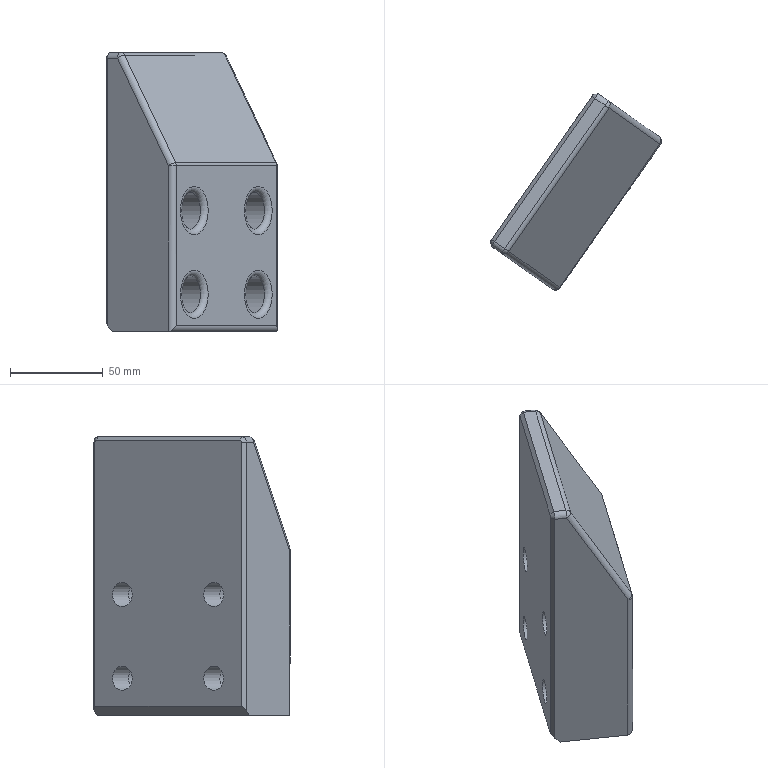Part | NX | features solid 2 | 1 solid | 42 faces | box 91.894 x 105.401 x 150 mm | volume 521981 mm3 | cylinder 17 | plane 15 | torus 4 | sphere 4 | cone 2 | commonest cylinder face diameters 6 x9 13 x4 20 x4
STEP:
#1=CARTESIAN_POINT('',(267.886,524.136,-269.059));
#2=VERTEX_POINT('',#1);
#3=CARTESIAN_POINT('',(260.429,513.487,-269.059));
#4=DIRECTION('',(0.8192,-0.5736,0.));
#5=DIRECTION('',(0.5736,0.8192,0.));
#6=AXIS2_PLACEMENT_3D('',#3,#4,#5);
#7=CIRCLE('',#6,13.);
#8=EDGE_CURVE('',#2,#2,#7,.F.);
#9=ORIENTED_EDGE('',*,*,#8,.T.);
#10=EDGE_LOOP('',(#9));
#11=FACE_BOUND('',#10,.T.);
#12=CARTESIAN_POINT('',(267.886,524.136,-314.059));
#13=VERTEX_POINT('',#12);
#14=CARTESIAN_POINT('',(260.429,513.487,-314.059));
#15=DIRECTION('',(0.8192,-0.5736,0.));
#16=DIRECTION('',(0.5736,0.8192,0.));
#17=AXIS2_PLACEMENT_3D('',#14,#15,#16);
#18=CIRCLE('',#17,13.);
#19=EDGE_CURVE('',#13,#13,#18,.F.);
#20=ORIENTED_EDGE('',*,*,#19,.T.);
#21=EDGE_LOOP('',(#20));
#22=FACE_BOUND('',#21,.T.);
#23=CARTESIAN_POINT('',(233.471,474.987,-269.059));
#24=VERTEX_POINT('',#23);
#25=CARTESIAN_POINT('',(226.015,464.338,-269.059));
#26=DIRECTION('',(0.8192,-0.5736,0.));
#27=DIRECTION('',(0.5736,0.8192,0.));
#28=AXIS2_PLACEMENT_3D('',#25,#26,#27);
#29=CIRCLE('',#28,13.);
#30=EDGE_CURVE('',#24,#24,#29,.F.);
#31=ORIENTED_EDGE('',*,*,#30,.T.);
#32=EDGE_LOOP('',(#31));
#33=FACE_BOUND('',#32,.T.);
#34=CARTESIAN_POINT('',(233.471,474.987,-314.059));
#35=VERTEX_POINT('',#34);
#36=CARTESIAN_POINT('',(226.015,464.338,-314.059));
#37=DIRECTION('',(0.8192,-0.5736,0.));
#38=DIRECTION('',(0.5736,0.8192,0.));
#39=AXIS2_PLACEMENT_3D('',#36,#37,#38);
#40=CIRCLE('',#39,13.);
#41=EDGE_CURVE('',#35,#35,#40,.F.);
#42=ORIENTED_EDGE('',*,*,#41,.T.);
#43=EDGE_LOOP('',(#42));
#44=FACE_BOUND('',#43,.T.);
#45=CARTESIAN_POINT('',(216.264,450.412,-244.863));
#46=VERTEX_POINT('',#45);
#47=CARTESIAN_POINT('',(216.264,450.412,-331.059));
#48=VERTEX_POINT('',#47);
#49=CARTESIAN_POINT('',(216.264,450.412,-334.059));
#50=DIRECTION('',(0.,0.,1.));
#51=VECTOR('',#50,1000.);
#52=LINE('',#49,#51);
#53=EDGE_CURVE('',#46,#48,#52,.F.);
#54=ORIENTED_EDGE('',*,*,#53,.T.);
#55=CARTESIAN_POINT('',(270.18,527.412,-331.059));
#56=VERTEX_POINT('',#55);
#57=CARTESIAN_POINT('',(271.901,529.87,-331.059));
#58=DIRECTION('',(-0.5736,-0.8192,0.));
#59=VECTOR('',#58,1000.);
#60=LINE('',#57,#59);
#61=EDGE_CURVE('',#48,#56,#60,.F.);
#62=ORIENTED_EDGE('',*,*,#61,.T.);
#63=CARTESIAN_POINT('',(270.18,527.412,-244.863));
#64=VERTEX_POINT('',#63);
#65=CARTESIAN_POINT('',(270.18,527.412,-244.059));
#66=DIRECTION('',(0.,0.,1.));
#67=VECTOR('',#66,1000.);
#68=LINE('',#65,#67);
#69=EDGE_CURVE('',#56,#64,#68,.T.);
#70=ORIENTED_EDGE('',*,*,#69,.T.);
#71=CARTESIAN_POINT('',(271.901,529.87,-244.863));
#72=DIRECTION('',(-0.5736,-0.8192,0.));
#73=VECTOR('',#72,1000.);
#74=LINE('',#71,#73);
#75=EDGE_CURVE('',#64,#46,#74,.T.);
#76=ORIENTED_EDGE('',*,*,#75,.T.);
#77=EDGE_LOOP('',(#54,#62,#70,#76));
#78=FACE_BOUND('',#77,.T.);
#79=CARTESIAN_POINT('',(271.901,529.87,-334.059));
#80=DIRECTION('',(0.8192,-0.5736,0.));
#81=DIRECTION('',(0.5736,0.8192,0.));
#82=AXIS2_PLACEMENT_3D('',#79,#80,#81);
#83=PLANE('',#82);
#84=ADVANCED_FACE('',(#11,#22,#33,#44,#78),#83,.T.);
#85=CARTESIAN_POINT('',(269.851,527.643,-243.363));
#86=VERTEX_POINT('',#85);
#87=CARTESIAN_POINT('',(242.513,546.785,-185.559));
#88=VERTEX_POINT('',#87);
#89=CARTESIAN_POINT('',(241.804,547.282,-184.059));
#90=DIRECTION('',(-0.4096,0.2868,0.866));
#91=VECTOR('',#90,1000.);
#92=LINE('',#89,#91);
#93=EDGE_CURVE('',#86,#88,#92,.T.);
#94=ORIENTED_EDGE('',*,*,#93,.T.);
#95=CARTESIAN_POINT('',(188.597,469.785,-185.559));
#96=VERTEX_POINT('',#95);
#97=CARTESIAN_POINT('',(244.234,549.242,-185.559));
#98=DIRECTION('',(-0.5736,-0.8192,0.));
#99=VECTOR('',#98,1000.);
#100=LINE('',#97,#99);
#101=EDGE_CURVE('',#88,#96,#100,.T.);
#102=ORIENTED_EDGE('',*,*,#101,.T.);
#103=CARTESIAN_POINT('',(215.935,450.643,-243.363));
#104=VERTEX_POINT('',#103);
#105=CARTESIAN_POINT('',(216.264,450.412,-244.059));
#106=DIRECTION('',(-0.4096,0.2868,0.866));
#107=VECTOR('',#106,1000.);
#108=LINE('',#105,#107);
#109=EDGE_CURVE('',#96,#104,#108,.F.);
#110=ORIENTED_EDGE('',*,*,#109,.T.);
#111=CARTESIAN_POINT('',(271.572,530.1,-243.363));
#112=DIRECTION('',(-0.5736,-0.8192,0.));
#113=VECTOR('',#112,1000.);
#114=LINE('',#111,#113);
#115=EDGE_CURVE('',#104,#86,#114,.F.);
#116=ORIENTED_EDGE('',*,*,#115,.T.);
#117=EDGE_LOOP('',(#94,#102,#110,#116));
#118=FACE_BOUND('',#117,.T.);
#119=CARTESIAN_POINT('',(271.901,529.87,-244.059));
#120=DIRECTION('',(0.7094,-0.4967,0.5));
#121=DIRECTION('',(0.4096,-0.2868,-0.866));
#122=AXIS2_PLACEMENT_3D('',#119,#120,#121);
#123=PLANE('',#122);
#124=ADVANCED_FACE('',(#118),#123,.T.);
#125=CARTESIAN_POINT('',(240.385,548.275,-184.059));
#126=VERTEX_POINT('',#125);
#127=CARTESIAN_POINT('',(234.957,552.076,-184.059));
#128=VERTEX_POINT('',#127);
#129=CARTESIAN_POINT('',(233.318,553.223,-184.059));
#130=DIRECTION('',(-0.8192,0.5736,0.));
#131=VECTOR('',#130,1000.);
#132=LINE('',#129,#131);
#133=EDGE_CURVE('',#126,#128,#132,.T.);
#134=ORIENTED_EDGE('',*,*,#133,.T.);
#135=CARTESIAN_POINT('',(181.041,475.076,-184.059));
#136=VERTEX_POINT('',#135);
#137=CARTESIAN_POINT('',(236.677,554.534,-184.059));
#138=DIRECTION('',(-0.5736,-0.8192,0.));
#139=VECTOR('',#138,1000.);
#140=LINE('',#137,#139);
#141=EDGE_CURVE('',#128,#136,#140,.T.);
#142=ORIENTED_EDGE('',*,*,#141,.T.);
#143=CARTESIAN_POINT('',(186.469,471.275,-184.059));
#144=VERTEX_POINT('',#143);
#145=CARTESIAN_POINT('',(187.888,470.281,-184.059));
#146=DIRECTION('',(-0.8192,0.5736,0.));
#147=VECTOR('',#146,1000.);
#148=LINE('',#145,#147);
#149=EDGE_CURVE('',#136,#144,#148,.F.);
#150=ORIENTED_EDGE('',*,*,#149,.T.);
#151=CARTESIAN_POINT('',(242.106,550.733,-184.059));
#152=DIRECTION('',(-0.5736,-0.8192,0.));
#153=VECTOR('',#152,1000.);
#154=LINE('',#151,#153);
#155=EDGE_CURVE('',#144,#126,#154,.F.);
#156=ORIENTED_EDGE('',*,*,#155,.T.);
#157=EDGE_LOOP('',(#134,#142,#150,#156));
#158=FACE_BOUND('',#157,.T.);
#159=CARTESIAN_POINT('',(243.525,549.739,-184.059));
#160=DIRECTION('',(0.,0.,1.));
#161=DIRECTION('',(-0.5736,-0.8192,0.));
#162=AXIS2_PLACEMENT_3D('',#159,#160,#161);
#163=PLANE('',#162);
#164=ADVANCED_FACE('',(#158),#163,.T.);
#165=CARTESIAN_POINT('',(219.839,533.973,-269.059));
#166=VERTEX_POINT('',#165);
#167=CARTESIAN_POINT('',(223.568,539.298,-269.059));
#168=DIRECTION('',(-0.8192,0.5736,0.));
#169=DIRECTION('',(-0.5736,-0.8192,0.));
#170=AXIS2_PLACEMENT_3D('',#167,#168,#169);
#171=CIRCLE('',#170,6.5);
#172=EDGE_CURVE('',#166,#166,#171,.T.);
#173=ORIENTED_EDGE('',*,*,#172,.F.);
#174=EDGE_LOOP('',(#173));
#175=FACE_BOUND('',#174,.T.);
#176=CARTESIAN_POINT('',(185.425,484.824,-269.059));
#177=VERTEX_POINT('',#176);
#178=CARTESIAN_POINT('',(189.153,490.149,-269.059));
#179=DIRECTION('',(-0.8192,0.5736,0.));
#180=DIRECTION('',(-0.5736,-0.8192,0.));
#181=AXIS2_PLACEMENT_3D('',#178,#179,#180);
#182=CIRCLE('',#181,6.5);
#183=EDGE_CURVE('',#177,#177,#182,.T.);
#184=ORIENTED_EDGE('',*,*,#183,.F.);
#185=EDGE_LOOP('',(#184));
#186=FACE_BOUND('',#185,.T.);
#187=CARTESIAN_POINT('',(219.839,533.973,-314.059));
#188=VERTEX_POINT('',#187);
#189=CARTESIAN_POINT('',(223.568,539.298,-314.059));
#190=DIRECTION('',(-0.8192,0.5736,0.));
#191=DIRECTION('',(-0.5736,-0.8192,0.));
#192=AXIS2_PLACEMENT_3D('',#189,#190,#191);
#193=CIRCLE('',#192,6.5);
#194=EDGE_CURVE('',#188,#188,#193,.T.);
#195=ORIENTED_EDGE('',*,*,#194,.F.);
#196=EDGE_LOOP('',(#195));
#197=FACE_BOUND('',#196,.T.);
#198=CARTESIAN_POINT('',(185.425,484.824,-314.059));
#199=VERTEX_POINT('',#198);
#200=CARTESIAN_POINT('',(189.153,490.149,-314.059));
#201=DIRECTION('',(-0.8192,0.5736,0.));
#202=DIRECTION('',(-0.5736,-0.8192,0.));
#203=AXIS2_PLACEMENT_3D('',#200,#201,#202);
#204=CIRCLE('',#203,6.5);
#205=EDGE_CURVE('',#199,#199,#204,.T.);
#206=ORIENTED_EDGE('',*,*,#205,.F.);
#207=EDGE_LOOP('',(#206));
#208=FACE_BOUND('',#207,.T.);
#209=CARTESIAN_POINT('',(233.892,554.043,-187.059));
#210=VERTEX_POINT('',#209);
#211=CARTESIAN_POINT('',(233.892,554.043,-329.059));
#212=VERTEX_POINT('',#211);
#213=CARTESIAN_POINT('',(233.892,554.043,-334.059));
#214=DIRECTION('',(0.,0.,-1.));
#215=VECTOR('',#214,1000.);
#216=LINE('',#213,#215);
#217=EDGE_CURVE('',#210,#212,#216,.T.);
#218=ORIENTED_EDGE('',*,*,#217,.T.);
#219=CARTESIAN_POINT('',(178.829,475.404,-329.059));
#220=VERTEX_POINT('',#219);
#221=CARTESIAN_POINT('',(235.039,555.681,-329.059));
#222=DIRECTION('',(-0.5736,-0.8192,0.));
#223=VECTOR('',#222,1000.);
#224=LINE('',#221,#223);
#225=EDGE_CURVE('',#212,#220,#224,.T.);
#226=ORIENTED_EDGE('',*,*,#225,.T.);
#227=CARTESIAN_POINT('',(178.829,475.404,-187.059));
#228=VERTEX_POINT('',#227);
#229=CARTESIAN_POINT('',(178.829,475.404,-184.059));
#230=DIRECTION('',(0.,0.,1.));
#231=VECTOR('',#230,1000.);
#232=LINE('',#229,#231);
#233=EDGE_CURVE('',#220,#228,#232,.T.);
#234=ORIENTED_EDGE('',*,*,#233,.T.);
#235=CARTESIAN_POINT('',(179.402,476.223,-186.059));
#236=VERTEX_POINT('',#235);
#237=CARTESIAN_POINT('',(179.402,476.223,-187.059));
#238=DIRECTION('',(-0.8192,0.5736,0.));
#239=DIRECTION('',(0.,0.,1.));
#240=AXIS2_PLACEMENT_3D('',#237,#238,#239);
#241=CIRCLE('',#240,1.);
#242=EDGE_CURVE('',#228,#236,#241,.T.);
#243=ORIENTED_EDGE('',*,*,#242,.T.);
#244=CARTESIAN_POINT('',(233.318,553.223,-186.059));
#245=VERTEX_POINT('',#244);
#246=CARTESIAN_POINT('',(235.039,555.681,-186.059));
#247=DIRECTION('',(0.5736,0.8192,0.));
#248=VECTOR('',#247,1000.);
#249=LINE('',#246,#248);
#250=EDGE_CURVE('',#236,#245,#249,.T.);
#251=ORIENTED_EDGE('',*,*,#250,.T.);
#252=CARTESIAN_POINT('',(233.318,553.223,-187.059));
#253=DIRECTION('',(-0.8192,0.5736,0.));
#254=DIRECTION('',(0.,0.,1.));
#255=AXIS2_PLACEMENT_3D('',#252,#253,#254);
#256=CIRCLE('',#255,1.);
#257=EDGE_CURVE('',#245,#210,#256,.T.);
#258=ORIENTED_EDGE('',*,*,#257,.T.);
#259=EDGE_LOOP('',(#218,#226,#234,#243,#251,#258));
#260=FACE_BOUND('',#259,.T.);
#261=CARTESIAN_POINT('',(235.039,555.681,-184.059));
#262=DIRECTION('',(-0.8192,0.5736,0.));
#263=DIRECTION('',(0.,0.,1.));
#264=AXIS2_PLACEMENT_3D('',#261,#262,#263);
#265=PLANE('',#264);
#266=ADVANCED_FACE('',(#175,#186,#197,#208,#260),#265,.T.);
#267=CARTESIAN_POINT('',(181.777,470.898,-334.059));
#268=VERTEX_POINT('',#267);
#269=CARTESIAN_POINT('',(212.086,449.675,-334.059));
#270=VERTEX_POINT('',#269);
#271=CARTESIAN_POINT('',(177.682,473.766,-334.059));
#272=DIRECTION('',(0.8192,-0.5736,0.));
#273=VECTOR('',#272,1000.);
#274=LINE('',#271,#273);
#275=EDGE_CURVE('',#268,#270,#274,.T.);
#276=ORIENTED_EDGE('',*,*,#275,.F.);
#277=CARTESIAN_POINT('',(239.135,552.813,-334.059));
#278=VERTEX_POINT('',#277);
#279=CARTESIAN_POINT('',(239.135,552.813,-334.059));
#280=DIRECTION('',(0.5736,0.8192,0.));
#281=VECTOR('',#280,1000.);
#282=LINE('',#279,#281);
#283=EDGE_CURVE('',#268,#278,#282,.T.);
#284=ORIENTED_EDGE('',*,*,#283,.T.);
#285=CARTESIAN_POINT('',(269.444,531.591,-334.059));
#286=VERTEX_POINT('',#285);
#287=CARTESIAN_POINT('',(235.039,555.681,-334.059));
#288=DIRECTION('',(0.8192,-0.5736,0.));
#289=VECTOR('',#288,1000.);
#290=LINE('',#287,#289);
#291=EDGE_CURVE('',#278,#286,#290,.T.);
#292=ORIENTED_EDGE('',*,*,#291,.T.);
#293=CARTESIAN_POINT('',(269.444,531.591,-334.059));
#294=DIRECTION('',(-0.5736,-0.8192,0.));
#295=VECTOR('',#294,1000.);
#296=LINE('',#293,#295);
#297=EDGE_CURVE('',#286,#270,#296,.T.);
#298=ORIENTED_EDGE('',*,*,#297,.T.);
#299=EDGE_LOOP('',(#276,#284,#292,#298));
#300=FACE_BOUND('',#299,.T.);
#301=CARTESIAN_POINT('',(235.039,555.681,-334.059));
#302=DIRECTION('',(0.,0.,-1.));
#303=DIRECTION('',(0.5736,0.8192,0.));
#304=AXIS2_PLACEMENT_3D('',#301,#302,#303);
#305=PLANE('',#304);
#306=ADVANCED_FACE('',(#300),#305,.T.);
#307=ORIENTED_EDGE('',*,*,#291,.F.);
#308=CARTESIAN_POINT('',(236.677,554.534,-331.059));
#309=VERTEX_POINT('',#308);
#310=CARTESIAN_POINT('',(235.039,555.681,-329.059));
#311=DIRECTION('',(0.5792,-0.4056,-0.7071));
#312=VECTOR('',#311,1000.);
#313=LINE('',#310,#312);
#314=EDGE_CURVE('',#278,#309,#313,.F.);
#315=ORIENTED_EDGE('',*,*,#314,.T.);
#316=CARTESIAN_POINT('',(236.677,554.534,-187.059));
#317=VERTEX_POINT('',#316);
#318=CARTESIAN_POINT('',(236.677,554.534,-187.059));
#319=DIRECTION('',(0.,0.,1.));
#320=VECTOR('',#319,1000.);
#321=LINE('',#318,#320);
#322=EDGE_CURVE('',#309,#317,#321,.T.);
#323=ORIENTED_EDGE('',*,*,#322,.T.);
#324=CARTESIAN_POINT('',(242.106,550.733,-187.059));
#325=VERTEX_POINT('',#324);
#326=CARTESIAN_POINT('',(243.525,549.739,-187.059));
#327=DIRECTION('',(-0.8192,0.5736,0.));
#328=VECTOR('',#327,1000.);
#329=LINE('',#326,#328);
#330=EDGE_CURVE('',#317,#325,#329,.F.);
#331=ORIENTED_EDGE('',*,*,#330,.T.);
#332=CARTESIAN_POINT('',(269.444,531.591,-244.863));
#333=VERTEX_POINT('',#332);
#334=CARTESIAN_POINT('',(269.773,531.36,-245.559));
#335=DIRECTION('',(-0.4096,0.2868,0.866));
#336=VECTOR('',#335,1000.);
#337=LINE('',#334,#336);
#338=EDGE_CURVE('',#325,#333,#337,.F.);
#339=ORIENTED_EDGE('',*,*,#338,.T.);
#340=CARTESIAN_POINT('',(269.444,531.591,-334.059));
#341=DIRECTION('',(0.,0.,1.));
#342=VECTOR('',#341,1000.);
#343=LINE('',#340,#342);
#344=EDGE_CURVE('',#333,#286,#343,.F.);
#345=ORIENTED_EDGE('',*,*,#344,.T.);
#346=EDGE_LOOP('',(#307,#315,#323,#331,#339,#345));
#347=FACE_BOUND('',#346,.T.);
#348=CARTESIAN_POINT('',(271.901,529.87,-184.059));
#349=DIRECTION('',(-0.5736,-0.8192,0.));
#350=DIRECTION('',(0.,0.,-1.));
#351=AXIS2_PLACEMENT_3D('',#348,#349,#350);
#352=PLANE('',#351);
#353=ADVANCED_FACE('',(#347),#352,.F.);
#354=CARTESIAN_POINT('',(179.32,472.618,-187.059));
#355=VERTEX_POINT('',#354);
#356=CARTESIAN_POINT('',(179.32,472.618,-331.059));
#357=VERTEX_POINT('',#356);
#358=CARTESIAN_POINT('',(179.32,472.618,-184.059));
#359=DIRECTION('',(0.,0.,-1.));
#360=VECTOR('',#359,1000.);
#361=LINE('',#358,#360);
#362=EDGE_CURVE('',#355,#357,#361,.T.);
#363=ORIENTED_EDGE('',*,*,#362,.T.);
#364=CARTESIAN_POINT('',(136.724,502.444,-279.059));
#365=DIRECTION('',(-0.5792,0.4056,0.7071));
#366=VECTOR('',#365,1000.);
#367=LINE('',#364,#366);
#368=EDGE_CURVE('',#357,#268,#367,.F.);
#369=ORIENTED_EDGE('',*,*,#368,.T.);
#370=ORIENTED_EDGE('',*,*,#275,.T.);
#371=CARTESIAN_POINT('',(212.086,449.675,-244.863));
#372=VERTEX_POINT('',#371);
#373=CARTESIAN_POINT('',(212.086,449.675,-184.059));
#374=DIRECTION('',(0.,0.,1.));
#375=VECTOR('',#374,1000.);
#376=LINE('',#373,#375);
#377=EDGE_CURVE('',#270,#372,#376,.T.);
#378=ORIENTED_EDGE('',*,*,#377,.T.);
#379=CARTESIAN_POINT('',(184.748,468.817,-187.059));
#380=VERTEX_POINT('',#379);
#381=CARTESIAN_POINT('',(191.133,464.347,-200.559));
#382=DIRECTION('',(-0.4096,0.2868,0.866));
#383=VECTOR('',#382,1000.);
#384=LINE('',#381,#383);
#385=EDGE_CURVE('',#372,#380,#384,.T.);
#386=ORIENTED_EDGE('',*,*,#385,.T.);
#387=CARTESIAN_POINT('',(214.543,447.955,-187.059));
#388=DIRECTION('',(-0.8192,0.5736,0.));
#389=VECTOR('',#388,1000.);
#390=LINE('',#387,#389);
#391=EDGE_CURVE('',#380,#355,#390,.T.);
#392=ORIENTED_EDGE('',*,*,#391,.T.);
#393=EDGE_LOOP('',(#363,#369,#370,#378,#386,#392));
#394=FACE_BOUND('',#393,.T.);
#395=CARTESIAN_POINT('',(214.543,447.955,-184.059));
#396=DIRECTION('',(-0.5736,-0.8192,0.));
#397=DIRECTION('',(0.,0.,-1.));
#398=AXIS2_PLACEMENT_3D('',#395,#396,#397);
#399=PLANE('',#398);
#400=ADVANCED_FACE('',(#394),#399,.T.);
#401=ORIENTED_EDGE('',*,*,#205,.T.);
#402=EDGE_LOOP('',(#401));
#403=FACE_BOUND('',#402,.T.);
#404=CARTESIAN_POINT('',(197.712,476.221,-314.059));
#405=VERTEX_POINT('',#404);
#406=CARTESIAN_POINT('',(201.44,481.545,-314.059));
#407=DIRECTION('',(-0.8192,0.5736,0.));
#408=DIRECTION('',(-0.5736,-0.8192,0.));
#409=AXIS2_PLACEMENT_3D('',#406,#407,#408);
#410=CIRCLE('',#409,6.5);
#411=EDGE_CURVE('',#405,#405,#410,.T.);
#412=ORIENTED_EDGE('',*,*,#411,.F.);
#413=EDGE_LOOP('',(#412));
#414=FACE_BOUND('',#413,.T.);
#415=CARTESIAN_POINT('',(189.153,490.149,-314.059));
#416=DIRECTION('',(-0.8192,0.5736,0.));
#417=DIRECTION('',(-0.5736,-0.8192,0.));
#418=AXIS2_PLACEMENT_3D('',#415,#416,#417);
#419=CYLINDRICAL_SURFACE('',#418,6.5);
#420=ADVANCED_FACE('',(#403,#414),#419,.F.);
#421=ORIENTED_EDGE('',*,*,#411,.T.);
#422=EDGE_LOOP('',(#421));
#423=FACE_BOUND('',#422,.T.);
#424=CARTESIAN_POINT('',(195.705,473.353,-314.059));
#425=VERTEX_POINT('',#424);
#426=CARTESIAN_POINT('',(201.44,481.545,-314.059));
#427=DIRECTION('',(-0.8192,0.5736,0.));
#428=DIRECTION('',(-0.5736,-0.8192,0.));
#429=AXIS2_PLACEMENT_3D('',#426,#427,#428);
#430=CIRCLE('',#429,10.);
#431=EDGE_CURVE('',#425,#425,#430,.T.);
#432=ORIENTED_EDGE('',*,*,#431,.F.);
#433=EDGE_LOOP('',(#432));
#434=FACE_BOUND('',#433,.T.);
#435=CARTESIAN_POINT('',(201.44,481.545,-314.059));
#436=DIRECTION('',(-0.8192,0.5736,0.));
#437=DIRECTION('',(-0.5736,-0.8192,0.));
#438=AXIS2_PLACEMENT_3D('',#435,#436,#437);
#439=PLANE('',#438);
#440=ADVANCED_FACE('',(#423,#434),#439,.F.);
#441=CARTESIAN_POINT('',(229.293,474.25,-314.059));
#442=VERTEX_POINT('',#441);
#443=CARTESIAN_POINT('',(223.557,466.058,-314.059));
#444=DIRECTION('',(0.8192,-0.5736,0.));
#445=DIRECTION('',(0.5736,0.8192,0.));
#446=AXIS2_PLACEMENT_3D('',#443,#444,#445);
#447=CIRCLE('',#446,10.);
#448=EDGE_CURVE('',#442,#442,#447,.T.);
#449=ORIENTED_EDGE('',*,*,#448,.T.);
#450=EDGE_LOOP('',(#449));
#451=FACE_BOUND('',#450,.T.);
#452=ORIENTED_EDGE('',*,*,#431,.T.);
#453=EDGE_LOOP('',(#452));
#454=FACE_BOUND('',#453,.T.);
#455=CARTESIAN_POINT('',(226.015,464.338,-314.059));
#456=DIRECTION('',(-0.8192,0.5736,0.));
#457=DIRECTION('',(-0.5736,-0.8192,0.));
#458=AXIS2_PLACEMENT_3D('',#455,#456,#457);
#459=CYLINDRICAL_SURFACE('',#458,10.);
#460=ADVANCED_FACE('',(#451,#454),#459,.F.);
#461=ORIENTED_EDGE('',*,*,#194,.T.);
#462=EDGE_LOOP('',(#461));
#463=FACE_BOUND('',#462,.T.);
#464=CARTESIAN_POINT('',(232.127,525.37,-314.059));
#465=VERTEX_POINT('',#464);
#466=CARTESIAN_POINT('',(235.855,530.694,-314.059));
#467=DIRECTION('',(-0.8192,0.5736,0.));
#468=DIRECTION('',(-0.5736,-0.8192,0.));
#469=AXIS2_PLACEMENT_3D('',#466,#467,#468);
#470=CIRCLE('',#469,6.5);
#471=EDGE_CURVE('',#465,#465,#470,.T.);
#472=ORIENTED_EDGE('',*,*,#471,.F.);
#473=EDGE_LOOP('',(#472));
#474=FACE_BOUND('',#473,.T.);
#475=CARTESIAN_POINT('',(223.568,539.298,-314.059));
#476=DIRECTION('',(-0.8192,0.5736,0.));
#477=DIRECTION('',(-0.5736,-0.8192,0.));
#478=AXIS2_PLACEMENT_3D('',#475,#476,#477);
#479=CYLINDRICAL_SURFACE('',#478,6.5);
#480=ADVANCED_FACE('',(#463,#474),#479,.F.);
#481=ORIENTED_EDGE('',*,*,#471,.T.);
#482=EDGE_LOOP('',(#481));
#483=FACE_BOUND('',#482,.T.);
#484=CARTESIAN_POINT('',(230.119,522.503,-314.059));
#485=VERTEX_POINT('',#484);
#486=CARTESIAN_POINT('',(235.855,530.694,-314.059));
#487=DIRECTION('',(-0.8192,0.5736,0.));
#488=DIRECTION('',(-0.5736,-0.8192,0.));
#489=AXIS2_PLACEMENT_3D('',#486,#487,#488);
#490=CIRCLE('',#489,10.);
#491=EDGE_CURVE('',#485,#485,#490,.T.);
#492=ORIENTED_EDGE('',*,*,#491,.F.);
#493=EDGE_LOOP('',(#492));
#494=FACE_BOUND('',#493,.T.);
#495=CARTESIAN_POINT('',(235.855,530.694,-314.059));
#496=DIRECTION('',(-0.8192,0.5736,0.));
#497=DIRECTION('',(-0.5736,-0.8192,0.));
#498=AXIS2_PLACEMENT_3D('',#495,#496,#497);
#499=PLANE('',#498);
#500=ADVANCED_FACE('',(#483,#494),#499,.F.);
#501=CARTESIAN_POINT('',(263.708,523.399,-314.059));
#502=VERTEX_POINT('',#501);
#503=CARTESIAN_POINT('',(257.972,515.208,-314.059));
#504=DIRECTION('',(0.8192,-0.5736,0.));
#505=DIRECTION('',(0.5736,0.8192,0.));
#506=AXIS2_PLACEMENT_3D('',#503,#504,#505);
#507=CIRCLE('',#506,10.);
#508=EDGE_CURVE('',#502,#502,#507,.T.);
#509=ORIENTED_EDGE('',*,*,#508,.T.);
#510=EDGE_LOOP('',(#509));
#511=FACE_BOUND('',#510,.T.);
#512=ORIENTED_EDGE('',*,*,#491,.T.);
#513=EDGE_LOOP('',(#512));
#514=FACE_BOUND('',#513,.T.);
#515=CARTESIAN_POINT('',(260.429,513.487,-314.059));
#516=DIRECTION('',(-0.8192,0.5736,0.));
#517=DIRECTION('',(-0.5736,-0.8192,0.));
#518=AXIS2_PLACEMENT_3D('',#515,#516,#517);
#519=CYLINDRICAL_SURFACE('',#518,10.);
#520=ADVANCED_FACE('',(#511,#514),#519,.F.);
#521=ORIENTED_EDGE('',*,*,#183,.T.);
#522=EDGE_LOOP('',(#521));
#523=FACE_BOUND('',#522,.T.);
#524=CARTESIAN_POINT('',(197.712,476.221,-269.059));
#525=VERTEX_POINT('',#524);
#526=CARTESIAN_POINT('',(201.44,481.545,-269.059));
#527=DIRECTION('',(-0.8192,0.5736,0.));
#528=DIRECTION('',(-0.5736,-0.8192,0.));
#529=AXIS2_PLACEMENT_3D('',#526,#527,#528);
#530=CIRCLE('',#529,6.5);
#531=EDGE_CURVE('',#525,#525,#530,.T.);
#532=ORIENTED_EDGE('',*,*,#531,.F.);
#533=EDGE_LOOP('',(#532));
#534=FACE_BOUND('',#533,.T.);
#535=CARTESIAN_POINT('',(189.153,490.149,-269.059));
#536=DIRECTION('',(-0.8192,0.5736,0.));
#537=DIRECTION('',(-0.5736,-0.8192,0.));
#538=AXIS2_PLACEMENT_3D('',#535,#536,#537);
#539=CYLINDRICAL_SURFACE('',#538,6.5);
#540=ADVANCED_FACE('',(#523,#534),#539,.F.);
#541=ORIENTED_EDGE('',*,*,#531,.T.);
#542=EDGE_LOOP('',(#541));
#543=FACE_BOUND('',#542,.T.);
#544=CARTESIAN_POINT('',(195.705,473.353,-269.059));
#545=VERTEX_POINT('',#544);
#546=CARTESIAN_POINT('',(201.44,481.545,-269.059));
#547=DIRECTION('',(-0.8192,0.5736,0.));
#548=DIRECTION('',(-0.5736,-0.8192,0.));
#549=AXIS2_PLACEMENT_3D('',#546,#547,#548);
#550=CIRCLE('',#549,10.);
#551=EDGE_CURVE('',#545,#545,#550,.T.);
#552=ORIENTED_EDGE('',*,*,#551,.F.);
#553=EDGE_LOOP('',(#552));
#554=FACE_BOUND('',#553,.T.);
#555=CARTESIAN_POINT('',(201.44,481.545,-269.059));
#556=DIRECTION('',(-0.8192,0.5736,0.));
#557=DIRECTION('',(-0.5736,-0.8192,0.));
#558=AXIS2_PLACEMENT_3D('',#555,#556,#557);
#559=PLANE('',#558);
#560=ADVANCED_FACE('',(#543,#554),#559,.F.);
#561=CARTESIAN_POINT('',(229.293,474.25,-269.059));
#562=VERTEX_POINT('',#561);
#563=CARTESIAN_POINT('',(223.557,466.058,-269.059));
#564=DIRECTION('',(0.8192,-0.5736,0.));
#565=DIRECTION('',(0.5736,0.8192,0.));
#566=AXIS2_PLACEMENT_3D('',#563,#564,#565);
#567=CIRCLE('',#566,10.);
#568=EDGE_CURVE('',#562,#562,#567,.T.);
#569=ORIENTED_EDGE('',*,*,#568,.T.);
#570=EDGE_LOOP('',(#569));
#571=FACE_BOUND('',#570,.T.);
#572=ORIENTED_EDGE('',*,*,#551,.T.);
#573=EDGE_LOOP('',(#572));
#574=FACE_BOUND('',#573,.T.);
#575=CARTESIAN_POINT('',(226.015,464.338,-269.059));
#576=DIRECTION('',(-0.8192,0.5736,0.));
#577=DIRECTION('',(-0.5736,-0.8192,0.));
#578=AXIS2_PLACEMENT_3D('',#575,#576,#577);
#579=CYLINDRICAL_SURFACE('',#578,10.);
#580=ADVANCED_FACE('',(#571,#574),#579,.F.);
#581=ORIENTED_EDGE('',*,*,#172,.T.);
#582=EDGE_LOOP('',(#581));
#583=FACE_BOUND('',#582,.T.);
#584=CARTESIAN_POINT('',(232.127,525.37,-269.059));
#585=VERTEX_POINT('',#584);
#586=CARTESIAN_POINT('',(235.855,530.694,-269.059));
#587=DIRECTION('',(-0.8192,0.5736,0.));
#588=DIRECTION('',(-0.5736,-0.8192,0.));
#589=AXIS2_PLACEMENT_3D('',#586,#587,#588);
#590=CIRCLE('',#589,6.5);
#591=EDGE_CURVE('',#585,#585,#590,.T.);
#592=ORIENTED_EDGE('',*,*,#591,.F.);
#593=EDGE_LOOP('',(#592));
#594=FACE_BOUND('',#593,.T.);
#595=CARTESIAN_POINT('',(223.568,539.298,-269.059));
#596=DIRECTION('',(-0.8192,0.5736,0.));
#597=DIRECTION('',(-0.5736,-0.8192,0.));
#598=AXIS2_PLACEMENT_3D('',#595,#596,#597);
#599=CYLINDRICAL_SURFACE('',#598,6.5);
#600=ADVANCED_FACE('',(#583,#594),#599,.F.);
#601=ORIENTED_EDGE('',*,*,#591,.T.);
#602=EDGE_LOOP('',(#601));
#603=FACE_BOUND('',#602,.T.);
#604=CARTESIAN_POINT('',(230.119,522.503,-269.059));
#605=VERTEX_POINT('',#604);
#606=CARTESIAN_POINT('',(235.855,530.694,-269.059));
#607=DIRECTION('',(-0.8192,0.5736,0.));
#608=DIRECTION('',(-0.5736,-0.8192,0.));
#609=AXIS2_PLACEMENT_3D('',#606,#607,#608);
#610=CIRCLE('',#609,10.);
#611=EDGE_CURVE('',#605,#605,#610,.T.);
#612=ORIENTED_EDGE('',*,*,#611,.F.);
#613=EDGE_LOOP('',(#612));
#614=FACE_BOUND('',#613,.T.);
#615=CARTESIAN_POINT('',(235.855,530.694,-269.059));
#616=DIRECTION('',(-0.8192,0.5736,0.));
#617=DIRECTION('',(-0.5736,-0.8192,0.));
#618=AXIS2_PLACEMENT_3D('',#615,#616,#617);
#619=PLANE('',#618);
#620=ADVANCED_FACE('',(#603,#614),#619,.F.);
#621=CARTESIAN_POINT('',(263.708,523.399,-269.059));
#622=VERTEX_POINT('',#621);
#623=CARTESIAN_POINT('',(257.972,515.208,-269.059));
#624=DIRECTION('',(0.8192,-0.5736,0.));
#625=DIRECTION('',(0.5736,0.8192,0.));
#626=AXIS2_PLACEMENT_3D('',#623,#624,#625);
#627=CIRCLE('',#626,10.);
#628=EDGE_CURVE('',#622,#622,#627,.T.);
#629=ORIENTED_EDGE('',*,*,#628,.T.);
#630=EDGE_LOOP('',(#629));
#631=FACE_BOUND('',#630,.T.);
#632=ORIENTED_EDGE('',*,*,#611,.T.);
#633=EDGE_LOOP('',(#632));
#634=FACE_BOUND('',#633,.T.);
#635=CARTESIAN_POINT('',(260.429,513.487,-269.059));
#636=DIRECTION('',(-0.8192,0.5736,0.));
#637=DIRECTION('',(-0.5736,-0.8192,0.));
#638=AXIS2_PLACEMENT_3D('',#635,#636,#637);
#639=CYLINDRICAL_SURFACE('',#638,10.);
#640=ADVANCED_FACE('',(#631,#634),#639,.F.);
#641=ORIENTED_EDGE('',*,*,#628,.F.);
#642=EDGE_LOOP('',(#641));
#643=FACE_BOUND('',#642,.T.);
#644=ORIENTED_EDGE('',*,*,#8,.F.);
#645=EDGE_LOOP('',(#644));
#646=FACE_BOUND('',#645,.T.);
#647=CARTESIAN_POINT('',(257.972,515.208,-269.059));
#648=DIRECTION('',(0.8192,-0.5736,0.));
#649=DIRECTION('',(0.5736,0.8192,0.));
#650=AXIS2_PLACEMENT_3D('',#647,#648,#649);
#651=TOROIDAL_SURFACE('',#650,13.,3.);
#652=ADVANCED_FACE('',(#643,#646),#651,.T.);
#653=ORIENTED_EDGE('',*,*,#508,.F.);
#654=EDGE_LOOP('',(#653));
#655=FACE_BOUND('',#654,.T.);
#656=ORIENTED_EDGE('',*,*,#19,.F.);
#657=EDGE_LOOP('',(#656));
#658=FACE_BOUND('',#657,.T.);
#659=CARTESIAN_POINT('',(257.972,515.208,-314.059));
#660=DIRECTION('',(0.8192,-0.5736,0.));
#661=DIRECTION('',(0.5736,0.8192,0.));
#662=AXIS2_PLACEMENT_3D('',#659,#660,#661);
#663=TOROIDAL_SURFACE('',#662,13.,3.);
#664=ADVANCED_FACE('',(#655,#658),#663,.T.);
#665=ORIENTED_EDGE('',*,*,#568,.F.);
#666=EDGE_LOOP('',(#665));
#667=FACE_BOUND('',#666,.T.);
#668=ORIENTED_EDGE('',*,*,#30,.F.);
#669=EDGE_LOOP('',(#668));
#670=FACE_BOUND('',#669,.T.);
#671=CARTESIAN_POINT('',(223.557,466.058,-269.059));
#672=DIRECTION('',(0.8192,-0.5736,0.));
#673=DIRECTION('',(0.5736,0.8192,0.));
#674=AXIS2_PLACEMENT_3D('',#671,#672,#673);
#675=TOROIDAL_SURFACE('',#674,13.,3.);
#676=ADVANCED_FACE('',(#667,#670),#675,.T.);
#677=ORIENTED_EDGE('',*,*,#448,.F.);
#678=EDGE_LOOP('',(#677));
#679=FACE_BOUND('',#678,.T.);
#680=ORIENTED_EDGE('',*,*,#41,.F.);
#681=EDGE_LOOP('',(#680));
#682=FACE_BOUND('',#681,.T.);
#683=CARTESIAN_POINT('',(223.557,466.058,-314.059));
#684=DIRECTION('',(0.8192,-0.5736,0.));
#685=DIRECTION('',(0.5736,0.8192,0.));
#686=AXIS2_PLACEMENT_3D('',#683,#684,#685);
#687=TOROIDAL_SURFACE('',#686,13.,3.);
#688=ADVANCED_FACE('',(#679,#682),#687,.T.);
#689=ORIENTED_EDGE('',*,*,#330,.F.);
#690=CARTESIAN_POINT('',(234.957,552.076,-187.059));
#691=DIRECTION('',(-0.8192,0.5736,0.));
#692=DIRECTION('',(-0.5736,-0.8192,0.));
#693=AXIS2_PLACEMENT_3D('',#690,#691,#692);
#694=CIRCLE('',#693,3.);
#695=EDGE_CURVE('',#317,#128,#694,.F.);
#696=ORIENTED_EDGE('',*,*,#695,.T.);
#697=ORIENTED_EDGE('',*,*,#133,.F.);
#698=CARTESIAN_POINT('',(240.385,548.275,-187.059));
#699=DIRECTION('',(0.8192,-0.5736,0.));
#700=DIRECTION('',(0.,0.,-1.));
#701=AXIS2_PLACEMENT_3D('',#698,#699,#700);
#702=CIRCLE('',#701,3.);
#703=EDGE_CURVE('',#325,#126,#702,.T.);
#704=ORIENTED_EDGE('',*,*,#703,.F.);
#705=EDGE_LOOP('',(#689,#696,#697,#704));
#706=FACE_BOUND('',#705,.T.);
#707=CARTESIAN_POINT('',(241.804,547.282,-187.059));
#708=DIRECTION('',(0.8192,-0.5736,0.));
#709=DIRECTION('',(0.5736,0.8192,0.));
#710=AXIS2_PLACEMENT_3D('',#707,#708,#709);
#711=CYLINDRICAL_SURFACE('',#710,3.);
#712=ADVANCED_FACE('',(#706),#711,.T.);
#713=CARTESIAN_POINT('',(240.385,548.275,-187.059));
#714=DIRECTION('',(-0.4096,0.2868,0.866));
#715=DIRECTION('',(0.7094,-0.4967,0.5));
#716=AXIS2_PLACEMENT_3D('',#713,#714,#715);
#717=CIRCLE('',#716,3.);
#718=EDGE_CURVE('',#325,#88,#717,.F.);
#719=ORIENTED_EDGE('',*,*,#718,.F.);
#720=ORIENTED_EDGE('',*,*,#703,.T.);
#721=CARTESIAN_POINT('',(240.385,548.275,-187.059));
#722=DIRECTION('',(0.5736,0.8192,0.));
#723=DIRECTION('',(0.,0.,1.));
#724=AXIS2_PLACEMENT_3D('',#721,#722,#723);
#725=CIRCLE('',#724,3.);
#726=EDGE_CURVE('',#88,#126,#725,.F.);
#727=ORIENTED_EDGE('',*,*,#726,.F.);
#728=EDGE_LOOP('',(#719,#720,#727));
#729=FACE_BOUND('',#728,.T.);
#730=CARTESIAN_POINT('',(240.385,548.275,-187.059));
#731=DIRECTION('',(0.5736,0.8192,0.));
#732=DIRECTION('',(0.,0.,1.));
#733=AXIS2_PLACEMENT_3D('',#730,#731,#732);
#734=SPHERICAL_SURFACE('',#733,3.);
#735=ADVANCED_FACE('',(#729),#734,.T.);
#736=ORIENTED_EDGE('',*,*,#149,.F.);
#737=CARTESIAN_POINT('',(181.041,475.076,-187.059));
#738=DIRECTION('',(-0.8192,0.5736,0.));
#739=DIRECTION('',(-0.5736,-0.8192,0.));
#740=AXIS2_PLACEMENT_3D('',#737,#738,#739);
#741=CIRCLE('',#740,3.);
#742=EDGE_CURVE('',#136,#355,#741,.F.);
#743=ORIENTED_EDGE('',*,*,#742,.T.);
#744=ORIENTED_EDGE('',*,*,#391,.F.);
#745=CARTESIAN_POINT('',(186.469,471.275,-187.059));
#746=DIRECTION('',(0.8192,-0.5736,0.));
#747=DIRECTION('',(0.5736,0.8192,0.));
#748=AXIS2_PLACEMENT_3D('',#745,#746,#747);
#749=CIRCLE('',#748,3.);
#750=EDGE_CURVE('',#144,#380,#749,.T.);
#751=ORIENTED_EDGE('',*,*,#750,.F.);
#752=EDGE_LOOP('',(#736,#743,#744,#751));
#753=FACE_BOUND('',#752,.T.);
#754=CARTESIAN_POINT('',(216.264,450.412,-187.059));
#755=DIRECTION('',(-0.8192,0.5736,0.));
#756=DIRECTION('',(-0.5736,-0.8192,0.));
#757=AXIS2_PLACEMENT_3D('',#754,#755,#756);
#758=CYLINDRICAL_SURFACE('',#757,3.);
#759=ADVANCED_FACE('',(#753),#758,.T.);
#760=ORIENTED_EDGE('',*,*,#726,.T.);
#761=ORIENTED_EDGE('',*,*,#155,.F.);
#762=CARTESIAN_POINT('',(186.469,471.275,-187.059));
#763=DIRECTION('',(-0.5736,-0.8192,0.));
#764=DIRECTION('',(0.,0.,-1.));
#765=AXIS2_PLACEMENT_3D('',#762,#763,#764);
#766=CIRCLE('',#765,3.);
#767=EDGE_CURVE('',#96,#144,#766,.T.);
#768=ORIENTED_EDGE('',*,*,#767,.F.);
#769=ORIENTED_EDGE('',*,*,#101,.F.);
#770=EDGE_LOOP('',(#760,#761,#768,#769));
#771=FACE_BOUND('',#770,.T.);
#772=CARTESIAN_POINT('',(242.106,550.733,-187.059));
#773=DIRECTION('',(-0.5736,-0.8192,0.));
#774=DIRECTION('',(0.,0.,-1.));
#775=AXIS2_PLACEMENT_3D('',#772,#773,#774);
#776=CYLINDRICAL_SURFACE('',#775,3.);
#777=ADVANCED_FACE('',(#771),#776,.T.);
#778=ORIENTED_EDGE('',*,*,#718,.T.);
#779=ORIENTED_EDGE('',*,*,#93,.F.);
#780=CARTESIAN_POINT('',(267.723,529.133,-244.863));
#781=DIRECTION('',(0.4096,-0.2868,-0.866));
#782=DIRECTION('',(-0.7094,0.4967,-0.5));
#783=AXIS2_PLACEMENT_3D('',#780,#781,#782);
#784=CIRCLE('',#783,3.);
#785=EDGE_CURVE('',#333,#86,#784,.T.);
#786=ORIENTED_EDGE('',*,*,#785,.F.);
#787=ORIENTED_EDGE('',*,*,#338,.F.);
#788=EDGE_LOOP('',(#778,#779,#786,#787));
#789=FACE_BOUND('',#788,.T.);
#790=CARTESIAN_POINT('',(268.052,528.903,-245.559));
#791=DIRECTION('',(0.4096,-0.2868,-0.866));
#792=DIRECTION('',(-0.7094,0.4967,-0.5));
#793=AXIS2_PLACEMENT_3D('',#790,#791,#792);
#794=CYLINDRICAL_SURFACE('',#793,3.);
#795=ADVANCED_FACE('',(#789),#794,.T.);
#796=ORIENTED_EDGE('',*,*,#767,.T.);
#797=ORIENTED_EDGE('',*,*,#750,.T.);
#798=CARTESIAN_POINT('',(186.469,471.275,-187.059));
#799=DIRECTION('',(-0.4096,0.2868,0.866));
#800=DIRECTION('',(0.7094,-0.4967,0.5));
#801=AXIS2_PLACEMENT_3D('',#798,#799,#800);
#802=CIRCLE('',#801,3.);
#803=EDGE_CURVE('',#96,#380,#802,.F.);
#804=ORIENTED_EDGE('',*,*,#803,.F.);
#805=EDGE_LOOP('',(#796,#797,#804));
#806=FACE_BOUND('',#805,.T.);
#807=CARTESIAN_POINT('',(186.469,471.275,-187.059));
#808=DIRECTION('',(0.5736,0.8192,0.));
#809=DIRECTION('',(0.,0.,1.));
#810=AXIS2_PLACEMENT_3D('',#807,#808,#809);
#811=SPHERICAL_SURFACE('',#810,3.);
#812=ADVANCED_FACE('',(#806),#811,.T.);
#813=CARTESIAN_POINT('',(267.723,529.133,-244.863));
#814=DIRECTION('',(0.5736,0.8192,0.));
#815=DIRECTION('',(0.,0.,1.));
#816=AXIS2_PLACEMENT_3D('',#813,#814,#815);
#817=CIRCLE('',#816,3.);
#818=EDGE_CURVE('',#64,#86,#817,.F.);
#819=ORIENTED_EDGE('',*,*,#818,.F.);
#820=CARTESIAN_POINT('',(267.723,529.133,-244.863));
#821=DIRECTION('',(0.,0.,1.));
#822=DIRECTION('',(-0.5736,-0.8192,0.));
#823=AXIS2_PLACEMENT_3D('',#820,#821,#822);
#824=CIRCLE('',#823,3.);
#825=EDGE_CURVE('',#333,#64,#824,.F.);
#826=ORIENTED_EDGE('',*,*,#825,.F.);
#827=ORIENTED_EDGE('',*,*,#785,.T.);
#828=EDGE_LOOP('',(#819,#826,#827));
#829=FACE_BOUND('',#828,.T.);
#830=CARTESIAN_POINT('',(267.723,529.133,-244.863));
#831=DIRECTION('',(0.5736,0.8192,0.));
#832=DIRECTION('',(0.,0.,1.));
#833=AXIS2_PLACEMENT_3D('',#830,#831,#832);
#834=SPHERICAL_SURFACE('',#833,3.);
#835=ADVANCED_FACE('',(#829),#834,.T.);
#836=ORIENTED_EDGE('',*,*,#825,.T.);
#837=ORIENTED_EDGE('',*,*,#69,.F.);
#838=CARTESIAN_POINT('',(267.723,529.133,-331.059));
#839=DIRECTION('',(-0.4056,-0.5792,-0.7071));
#840=DIRECTION('',(-0.4056,-0.5792,0.7071));
#841=AXIS2_PLACEMENT_3D('',#838,#839,#840);
#842=ELLIPSE('',#841,4.243,3.);
#843=EDGE_CURVE('',#286,#56,#842,.T.);
#844=ORIENTED_EDGE('',*,*,#843,.F.);
#845=ORIENTED_EDGE('',*,*,#344,.F.);
#846=EDGE_LOOP('',(#836,#837,#844,#845));
#847=FACE_BOUND('',#846,.T.);
#848=CARTESIAN_POINT('',(267.723,529.133,-334.059));
#849=DIRECTION('',(0.,0.,-1.));
#850=DIRECTION('',(0.5736,0.8192,0.));
#851=AXIS2_PLACEMENT_3D('',#848,#849,#850);
#852=CYLINDRICAL_SURFACE('',#851,3.);
#853=ADVANCED_FACE('',(#847),#852,.T.);
#854=ORIENTED_EDGE('',*,*,#803,.T.);
#855=ORIENTED_EDGE('',*,*,#385,.F.);
#856=CARTESIAN_POINT('',(213.807,452.133,-244.863));
#857=DIRECTION('',(0.4096,-0.2868,-0.866));
#858=DIRECTION('',(-0.7094,0.4967,-0.5));
#859=AXIS2_PLACEMENT_3D('',#856,#857,#858);
#860=CIRCLE('',#859,3.);
#861=EDGE_CURVE('',#104,#372,#860,.T.);
#862=ORIENTED_EDGE('',*,*,#861,.F.);
#863=ORIENTED_EDGE('',*,*,#109,.F.);
#864=EDGE_LOOP('',(#854,#855,#862,#863));
#865=FACE_BOUND('',#864,.T.);
#866=CARTESIAN_POINT('',(192.854,466.804,-200.559));
#867=DIRECTION('',(-0.4096,0.2868,0.866));
#868=DIRECTION('',(0.7094,-0.4967,0.5));
#869=AXIS2_PLACEMENT_3D('',#866,#867,#868);
#870=CYLINDRICAL_SURFACE('',#869,3.);
#871=ADVANCED_FACE('',(#865),#870,.T.);
#872=ORIENTED_EDGE('',*,*,#818,.T.);
#873=ORIENTED_EDGE('',*,*,#115,.F.);
#874=CARTESIAN_POINT('',(213.807,452.133,-244.863));
#875=DIRECTION('',(-0.5736,-0.8192,0.));
#876=DIRECTION('',(0.,0.,-1.));
#877=AXIS2_PLACEMENT_3D('',#874,#875,#876);
#878=CIRCLE('',#877,3.);
#879=EDGE_CURVE('',#46,#104,#878,.T.);
#880=ORIENTED_EDGE('',*,*,#879,.F.);
#881=ORIENTED_EDGE('',*,*,#75,.F.);
#882=EDGE_LOOP('',(#872,#873,#880,#881));
#883=FACE_BOUND('',#882,.T.);
#884=CARTESIAN_POINT('',(269.444,531.591,-244.863));
#885=DIRECTION('',(-0.5736,-0.8192,0.));
#886=DIRECTION('',(0.,0.,-1.));
#887=AXIS2_PLACEMENT_3D('',#884,#885,#886);
#888=CYLINDRICAL_SURFACE('',#887,3.);
#889=ADVANCED_FACE('',(#883),#888,.T.);
#890=ORIENTED_EDGE('',*,*,#843,.T.);
#891=ORIENTED_EDGE('',*,*,#61,.F.);
#892=CARTESIAN_POINT('',(213.807,452.133,-331.059));
#893=DIRECTION('',(-0.4056,-0.5792,0.7071));
#894=DIRECTION('',(-0.4056,-0.5792,-0.7071));
#895=AXIS2_PLACEMENT_3D('',#892,#893,#894);
#896=ELLIPSE('',#895,4.243,3.);
#897=EDGE_CURVE('',#270,#48,#896,.T.);
#898=ORIENTED_EDGE('',*,*,#897,.F.);
#899=ORIENTED_EDGE('',*,*,#297,.F.);
#900=EDGE_LOOP('',(#890,#891,#898,#899));
#901=FACE_BOUND('',#900,.T.);
#902=CARTESIAN_POINT('',(269.444,531.591,-331.059));
#903=DIRECTION('',(-0.5736,-0.8192,0.));
#904=DIRECTION('',(0.,0.,-1.));
#905=AXIS2_PLACEMENT_3D('',#902,#903,#904);
#906=CYLINDRICAL_SURFACE('',#905,3.);
#907=ADVANCED_FACE('',(#901),#906,.T.);
#908=ORIENTED_EDGE('',*,*,#879,.T.);
#909=ORIENTED_EDGE('',*,*,#861,.T.);
#910=CARTESIAN_POINT('',(213.807,452.133,-244.863));
#911=DIRECTION('',(0.,0.,1.));
#912=DIRECTION('',(0.8192,-0.5736,0.));
#913=AXIS2_PLACEMENT_3D('',#910,#911,#912);
#914=CIRCLE('',#913,3.);
#915=EDGE_CURVE('',#46,#372,#914,.F.);
#916=ORIENTED_EDGE('',*,*,#915,.F.);
#917=EDGE_LOOP('',(#908,#909,#916));
#918=FACE_BOUND('',#917,.T.);
#919=CARTESIAN_POINT('',(213.807,452.133,-244.863));
#920=DIRECTION('',(0.5736,0.8192,0.));
#921=DIRECTION('',(0.,0.,1.));
#922=AXIS2_PLACEMENT_3D('',#919,#920,#921);
#923=SPHERICAL_SURFACE('',#922,3.);
#924=ADVANCED_FACE('',(#918),#923,.T.);
#925=ORIENTED_EDGE('',*,*,#897,.T.);
#926=ORIENTED_EDGE('',*,*,#53,.F.);
#927=ORIENTED_EDGE('',*,*,#915,.T.);
#928=ORIENTED_EDGE('',*,*,#377,.F.);
#929=EDGE_LOOP('',(#925,#926,#927,#928));
#930=FACE_BOUND('',#929,.T.);
#931=CARTESIAN_POINT('',(213.807,452.133,-184.059));
#932=DIRECTION('',(0.,0.,1.));
#933=DIRECTION('',(-0.5736,-0.8192,0.));
#934=AXIS2_PLACEMENT_3D('',#931,#932,#933);
#935=CYLINDRICAL_SURFACE('',#934,3.);
#936=ADVANCED_FACE('',(#930),#935,.T.);
#937=ORIENTED_EDGE('',*,*,#322,.F.);
#938=CARTESIAN_POINT('',(166.577,542.173,-280.725));
#939=DIRECTION('',(0.8041,0.1418,-0.5774));
#940=VECTOR('',#939,1000.);
#941=LINE('',#938,#940);
#942=EDGE_CURVE('',#309,#212,#941,.F.);
#943=ORIENTED_EDGE('',*,*,#942,.T.);
#944=ORIENTED_EDGE('',*,*,#217,.F.);
#945=CARTESIAN_POINT('',(236.677,554.534,-187.059));
#946=DIRECTION('',(-0.9848,-0.1736,0.));
#947=VECTOR('',#946,1000.);
#948=LINE('',#945,#947);
#949=EDGE_CURVE('',#317,#210,#948,.T.);
#950=ORIENTED_EDGE('',*,*,#949,.F.);
#951=EDGE_LOOP('',(#937,#943,#944,#950));
#952=FACE_BOUND('',#951,.T.);
#953=CARTESIAN_POINT('',(233.892,554.043,-184.059));
#954=DIRECTION('',(-0.1736,0.9848,0.));
#955=DIRECTION('',(-0.9848,-0.1736,0.));
#956=AXIS2_PLACEMENT_3D('',#953,#954,#955);
#957=PLANE('',#956);
#958=ADVANCED_FACE('',(#952),#957,.T.);
#959=ORIENTED_EDGE('',*,*,#949,.T.);
#960=ORIENTED_EDGE('',*,*,#257,.F.);
#961=CARTESIAN_POINT('',(234.957,552.076,-184.059));
#962=DIRECTION('',(-0.5792,0.4056,-0.7071));
#963=VECTOR('',#962,1000.);
#964=LINE('',#961,#963);
#965=EDGE_CURVE('',#128,#245,#964,.T.);
#966=ORIENTED_EDGE('',*,*,#965,.F.);
#967=ORIENTED_EDGE('',*,*,#695,.F.);
#968=EDGE_LOOP('',(#959,#960,#966,#967));
#969=FACE_BOUND('',#968,.T.);
#970=CARTESIAN_POINT('',(233.318,553.223,-187.059));
#971=DIRECTION('',(0.8192,-0.5736,0.));
#972=DIRECTION('',(0.5736,0.8192,0.));
#973=AXIS2_PLACEMENT_3D('',#970,#971,#972);
#974=CONICAL_SURFACE('',#973,1.,0.7854);
#975=ADVANCED_FACE('',(#969),#974,.T.);
#976=ORIENTED_EDGE('',*,*,#965,.T.);
#977=ORIENTED_EDGE('',*,*,#250,.F.);
#978=CARTESIAN_POINT('',(181.041,475.076,-184.059));
#979=DIRECTION('',(-0.5792,0.4056,-0.7071));
#980=VECTOR('',#979,1000.);
#981=LINE('',#978,#980);
#982=EDGE_CURVE('',#136,#236,#981,.T.);
#983=ORIENTED_EDGE('',*,*,#982,.F.);
#984=ORIENTED_EDGE('',*,*,#141,.F.);
#985=EDGE_LOOP('',(#976,#977,#983,#984));
#986=FACE_BOUND('',#985,.T.);
#987=CARTESIAN_POINT('',(236.677,554.534,-184.059));
#988=DIRECTION('',(0.5792,-0.4056,-0.7071));
#989=DIRECTION('',(-0.5792,0.4056,-0.7071));
#990=AXIS2_PLACEMENT_3D('',#987,#988,#989);
#991=PLANE('',#990);
#992=ADVANCED_FACE('',(#986),#991,.F.);
#993=ORIENTED_EDGE('',*,*,#982,.T.);
#994=ORIENTED_EDGE('',*,*,#242,.F.);
#995=CARTESIAN_POINT('',(179.32,472.618,-187.059));
#996=DIRECTION('',(-0.1736,0.9848,0.));
#997=VECTOR('',#996,1000.);
#998=LINE('',#995,#997);
#999=EDGE_CURVE('',#355,#228,#998,.T.);
#1000=ORIENTED_EDGE('',*,*,#999,.F.);
#1001=ORIENTED_EDGE('',*,*,#742,.F.);
#1002=EDGE_LOOP('',(#993,#994,#1000,#1001));
#1003=FACE_BOUND('',#1002,.T.);
#1004=CARTESIAN_POINT('',(179.402,476.223,-187.059));
#1005=DIRECTION('',(0.8192,-0.5736,0.));
#1006=DIRECTION('',(0.5736,0.8192,0.));
#1007=AXIS2_PLACEMENT_3D('',#1004,#1005,#1006);
#1008=CONICAL_SURFACE('',#1007,1.,0.7854);
#1009=ADVANCED_FACE('',(#1003),#1008,.T.);
#1010=ORIENTED_EDGE('',*,*,#233,.F.);
#1011=CARTESIAN_POINT('',(167.287,540.862,-282.059));
#1012=DIRECTION('',(0.1418,-0.8041,-0.5774));
#1013=VECTOR('',#1012,1000.);
#1014=LINE('',#1011,#1013);
#1015=EDGE_CURVE('',#220,#357,#1014,.T.);
#1016=ORIENTED_EDGE('',*,*,#1015,.T.);
#1017=ORIENTED_EDGE('',*,*,#362,.F.);
#1018=ORIENTED_EDGE('',*,*,#999,.T.);
#1019=EDGE_LOOP('',(#1010,#1016,#1017,#1018));
#1020=FACE_BOUND('',#1019,.T.);
#1021=CARTESIAN_POINT('',(179.32,472.618,-184.059));
#1022=DIRECTION('',(0.9848,0.1736,0.));
#1023=DIRECTION('',(-0.1736,0.9848,0.));
#1024=AXIS2_PLACEMENT_3D('',#1021,#1022,#1023);
#1025=PLANE('',#1024);
#1026=ADVANCED_FACE('',(#1020),#1025,.F.);
#1027=ORIENTED_EDGE('',*,*,#314,.F.);
#1028=ORIENTED_EDGE('',*,*,#283,.F.);
#1029=ORIENTED_EDGE('',*,*,#368,.F.);
#1030=ORIENTED_EDGE('',*,*,#1015,.F.);
#1031=ORIENTED_EDGE('',*,*,#225,.F.);
#1032=ORIENTED_EDGE('',*,*,#942,.F.);
#1033=EDGE_LOOP('',(#1027,#1028,#1029,#1030,#1031,#1032));
#1034=FACE_BOUND('',#1033,.T.);
#1035=CARTESIAN_POINT('',(235.039,555.681,-329.059));
#1036=DIRECTION('',(0.5792,-0.4056,0.7071));
#1037=DIRECTION('',(0.5792,-0.4056,-0.7071));
#1038=AXIS2_PLACEMENT_3D('',#1035,#1036,#1037);
#1039=PLANE('',#1038);
#1040=ADVANCED_FACE('',(#1034),#1039,.F.);
#1041=CLOSED_SHELL('',(#84,#124,#164,#266,#306,#353,#400,#420,#440,#460,#480,#500,#520,#540,#560,#580,#600,#620,#640,#652,#664,#676,#688,#712,#735,#759,#777,#795,#812,#835,#853,#871,#889,#907,#924,#936,#958,#975,#992,#1009,#1026,#1040));
#1042=MANIFOLD_SOLID_BREP('',#1041);
#1043=(LENGTH_UNIT()NAMED_UNIT(*)SI_UNIT(.MILLI.,.METRE.));
#1044=UNCERTAINTY_MEASURE_WITH_UNIT(LENGTH_MEASURE(0.00001),#1043,'','');
#1045=(NAMED_UNIT(*)PLANE_ANGLE_UNIT()SI_UNIT($,.RADIAN.));
#1046=(NAMED_UNIT(*)SI_UNIT($,.STERADIAN.)SOLID_ANGLE_UNIT());
#1047=(GEOMETRIC_REPRESENTATION_CONTEXT(3)GLOBAL_UNCERTAINTY_ASSIGNED_CONTEXT((#1044))GLOBAL_UNIT_ASSIGNED_CONTEXT((#1043,#1045,#1046))REPRESENTATION_CONTEXT('',''));
#1048=ADVANCED_BREP_SHAPE_REPRESENTATION('',(#1042),#1047);